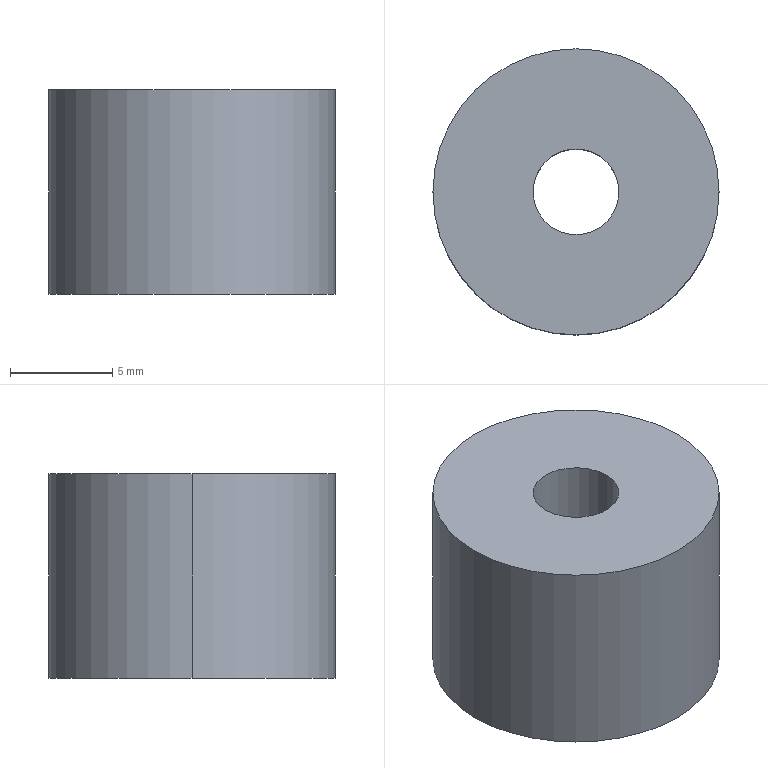Part | SolidWorks | features Extrusion 1, HoleWzd 1 | 1 solid | 6 faces | box 14 x 14 x 10 mm | volume 1401 mm3 | cylinder 4 | plane 2 | commonest cylinder face diameters 4.2 x2 14 x2
STEP:
#1=CARTESIAN_POINT('',(-2.1,0.,0.));
#2=VERTEX_POINT('',#1);
#3=CARTESIAN_POINT('',(2.1,0.,0.));
#4=VERTEX_POINT('',#3);
#5=CARTESIAN_POINT('',(0.,0.,0.));
#6=DIRECTION('',(0.,0.,1.));
#7=DIRECTION('',(1.,0.,0.));
#8=AXIS2_PLACEMENT_3D('',#5,#6,#7);
#9=CIRCLE('',#8,2.1);
#10=EDGE_CURVE('',#2,#4,#9,.T.);
#11=ORIENTED_EDGE('',*,*,#10,.F.);
#12=CARTESIAN_POINT('',(-2.1,0.,10.));
#13=VERTEX_POINT('',#12);
#14=CARTESIAN_POINT('',(-2.1,0.,10.));
#15=DIRECTION('',(0.,0.,1.));
#16=VECTOR('',#15,1000.);
#17=LINE('',#14,#16);
#18=EDGE_CURVE('',#2,#13,#17,.T.);
#19=ORIENTED_EDGE('',*,*,#18,.T.);
#20=CARTESIAN_POINT('',(2.1,0.,10.));
#21=VERTEX_POINT('',#20);
#22=CARTESIAN_POINT('',(0.,0.,10.));
#23=DIRECTION('',(0.,0.,1.));
#24=DIRECTION('',(1.,0.,0.));
#25=AXIS2_PLACEMENT_3D('',#22,#23,#24);
#26=CIRCLE('',#25,2.1);
#27=EDGE_CURVE('',#13,#21,#26,.T.);
#28=ORIENTED_EDGE('',*,*,#27,.T.);
#29=CARTESIAN_POINT('',(2.1,0.,10.));
#30=DIRECTION('',(0.,0.,1.));
#31=VECTOR('',#30,1000.);
#32=LINE('',#29,#31);
#33=EDGE_CURVE('',#4,#21,#32,.T.);
#34=ORIENTED_EDGE('',*,*,#33,.F.);
#35=EDGE_LOOP('',(#11,#19,#28,#34));
#36=FACE_OUTER_BOUND('',#35,.T.);
#37=CARTESIAN_POINT('',(0.,0.,10.));
#38=DIRECTION('',(0.,0.,1.));
#39=DIRECTION('',(1.,0.,0.));
#40=AXIS2_PLACEMENT_3D('',#37,#38,#39);
#41=CYLINDRICAL_SURFACE('',#40,2.1);
#42=ADVANCED_FACE('',(#36),#41,.F.);
#43=CARTESIAN_POINT('',(7.,0.,10.));
#44=VERTEX_POINT('',#43);
#45=CARTESIAN_POINT('',(-7.,0.,10.));
#46=VERTEX_POINT('',#45);
#47=CARTESIAN_POINT('',(0.,0.,10.));
#48=DIRECTION('',(0.,0.,1.));
#49=DIRECTION('',(1.,0.,0.));
#50=AXIS2_PLACEMENT_3D('',#47,#48,#49);
#51=CIRCLE('',#50,7.);
#52=EDGE_CURVE('',#44,#46,#51,.T.);
#53=ORIENTED_EDGE('',*,*,#52,.F.);
#54=CARTESIAN_POINT('',(7.,0.,0.));
#55=VERTEX_POINT('',#54);
#56=CARTESIAN_POINT('',(7.,0.,10.));
#57=DIRECTION('',(0.,0.,-1.));
#58=VECTOR('',#57,1000.);
#59=LINE('',#56,#58);
#60=EDGE_CURVE('',#44,#55,#59,.T.);
#61=ORIENTED_EDGE('',*,*,#60,.T.);
#62=CARTESIAN_POINT('',(-7.,0.,0.));
#63=VERTEX_POINT('',#62);
#64=CARTESIAN_POINT('',(0.,0.,0.));
#65=DIRECTION('',(0.,0.,1.));
#66=DIRECTION('',(1.,0.,0.));
#67=AXIS2_PLACEMENT_3D('',#64,#65,#66);
#68=CIRCLE('',#67,7.);
#69=EDGE_CURVE('',#55,#63,#68,.T.);
#70=ORIENTED_EDGE('',*,*,#69,.T.);
#71=CARTESIAN_POINT('',(-7.,0.,10.));
#72=DIRECTION('',(0.,0.,-1.));
#73=VECTOR('',#72,1000.);
#74=LINE('',#71,#73);
#75=EDGE_CURVE('',#46,#63,#74,.T.);
#76=ORIENTED_EDGE('',*,*,#75,.F.);
#77=EDGE_LOOP('',(#53,#61,#70,#76));
#78=FACE_OUTER_BOUND('',#77,.T.);
#79=CARTESIAN_POINT('',(0.,0.,10.));
#80=DIRECTION('',(0.,0.,-1.));
#81=DIRECTION('',(-1.,0.,0.));
#82=AXIS2_PLACEMENT_3D('',#79,#80,#81);
#83=CYLINDRICAL_SURFACE('',#82,7.);
#84=ADVANCED_FACE('',(#78),#83,.T.);
#85=ORIENTED_EDGE('',*,*,#60,.F.);
#86=CARTESIAN_POINT('',(0.,0.,10.));
#87=DIRECTION('',(0.,0.,1.));
#88=DIRECTION('',(1.,0.,0.));
#89=AXIS2_PLACEMENT_3D('',#86,#87,#88);
#90=CIRCLE('',#89,7.);
#91=EDGE_CURVE('',#46,#44,#90,.T.);
#92=ORIENTED_EDGE('',*,*,#91,.F.);
#93=ORIENTED_EDGE('',*,*,#75,.T.);
#94=CARTESIAN_POINT('',(0.,0.,0.));
#95=DIRECTION('',(0.,0.,1.));
#96=DIRECTION('',(1.,0.,0.));
#97=AXIS2_PLACEMENT_3D('',#94,#95,#96);
#98=CIRCLE('',#97,7.);
#99=EDGE_CURVE('',#63,#55,#98,.T.);
#100=ORIENTED_EDGE('',*,*,#99,.T.);
#101=EDGE_LOOP('',(#85,#92,#93,#100));
#102=FACE_OUTER_BOUND('',#101,.T.);
#103=CARTESIAN_POINT('',(0.,0.,10.));
#104=DIRECTION('',(0.,0.,-1.));
#105=DIRECTION('',(-1.,0.,0.));
#106=AXIS2_PLACEMENT_3D('',#103,#104,#105);
#107=CYLINDRICAL_SURFACE('',#106,7.);
#108=ADVANCED_FACE('',(#102),#107,.T.);
#109=CARTESIAN_POINT('',(0.,0.,10.));
#110=DIRECTION('',(0.,0.,1.));
#111=DIRECTION('',(1.,0.,0.));
#112=AXIS2_PLACEMENT_3D('',#109,#110,#111);
#113=CIRCLE('',#112,2.1);
#114=EDGE_CURVE('',#21,#13,#113,.T.);
#115=ORIENTED_EDGE('',*,*,#114,.F.);
#116=ORIENTED_EDGE('',*,*,#27,.F.);
#117=EDGE_LOOP('',(#115,#116));
#118=FACE_BOUND('',#117,.T.);
#119=ORIENTED_EDGE('',*,*,#91,.T.);
#120=ORIENTED_EDGE('',*,*,#52,.T.);
#121=EDGE_LOOP('',(#119,#120));
#122=FACE_OUTER_BOUND('',#121,.T.);
#123=CARTESIAN_POINT('',(0.,0.,10.));
#124=DIRECTION('',(0.,0.,1.));
#125=DIRECTION('',(1.,0.,0.));
#126=AXIS2_PLACEMENT_3D('',#123,#124,#125);
#127=PLANE('',#126);
#128=ADVANCED_FACE('',(#118,#122),#127,.T.);
#129=CARTESIAN_POINT('',(0.,0.,0.));
#130=DIRECTION('',(0.,0.,1.));
#131=DIRECTION('',(1.,0.,0.));
#132=AXIS2_PLACEMENT_3D('',#129,#130,#131);
#133=CIRCLE('',#132,2.1);
#134=EDGE_CURVE('',#4,#2,#133,.T.);
#135=ORIENTED_EDGE('',*,*,#134,.T.);
#136=ORIENTED_EDGE('',*,*,#10,.T.);
#137=EDGE_LOOP('',(#135,#136));
#138=FACE_BOUND('',#137,.T.);
#139=ORIENTED_EDGE('',*,*,#99,.F.);
#140=ORIENTED_EDGE('',*,*,#69,.F.);
#141=EDGE_LOOP('',(#139,#140));
#142=FACE_OUTER_BOUND('',#141,.T.);
#143=CARTESIAN_POINT('',(0.,0.,0.));
#144=DIRECTION('',(0.,0.,1.));
#145=DIRECTION('',(1.,0.,0.));
#146=AXIS2_PLACEMENT_3D('',#143,#144,#145);
#147=PLANE('',#146);
#148=ADVANCED_FACE('',(#138,#142),#147,.F.);
#149=ORIENTED_EDGE('',*,*,#18,.F.);
#150=ORIENTED_EDGE('',*,*,#134,.F.);
#151=ORIENTED_EDGE('',*,*,#33,.T.);
#152=ORIENTED_EDGE('',*,*,#114,.T.);
#153=EDGE_LOOP('',(#149,#150,#151,#152));
#154=FACE_OUTER_BOUND('',#153,.T.);
#155=CARTESIAN_POINT('',(0.,0.,10.));
#156=DIRECTION('',(0.,0.,1.));
#157=DIRECTION('',(1.,0.,0.));
#158=AXIS2_PLACEMENT_3D('',#155,#156,#157);
#159=CYLINDRICAL_SURFACE('',#158,2.1);
#160=ADVANCED_FACE('',(#154),#159,.F.);
#161=CLOSED_SHELL('',(#42,#84,#108,#128,#148,#160));
#162=MANIFOLD_SOLID_BREP('',#161);
#163=CARTESIAN_POINT('',(0.,0.,0.));
#164=DIRECTION('',(0.,0.,1.));
#165=DIRECTION('',(1.,0.,0.));
#166=AXIS2_PLACEMENT_3D('',#163,#164,#165);
#167=(LENGTH_UNIT()NAMED_UNIT(*)SI_UNIT(.MILLI.,.METRE.));
#168=UNCERTAINTY_MEASURE_WITH_UNIT(LENGTH_MEASURE(0.00001),#167,'','');
#169=(NAMED_UNIT(*)PLANE_ANGLE_UNIT()SI_UNIT($,.RADIAN.));
#170=(NAMED_UNIT(*)SI_UNIT($,.STERADIAN.)SOLID_ANGLE_UNIT());
#171=(GEOMETRIC_REPRESENTATION_CONTEXT(3)GLOBAL_UNCERTAINTY_ASSIGNED_CONTEXT((#168))GLOBAL_UNIT_ASSIGNED_CONTEXT((#167,#169,#170))REPRESENTATION_CONTEXT('',''));
#172=ADVANCED_BREP_SHAPE_REPRESENTATION('',(#162,#166),#171);